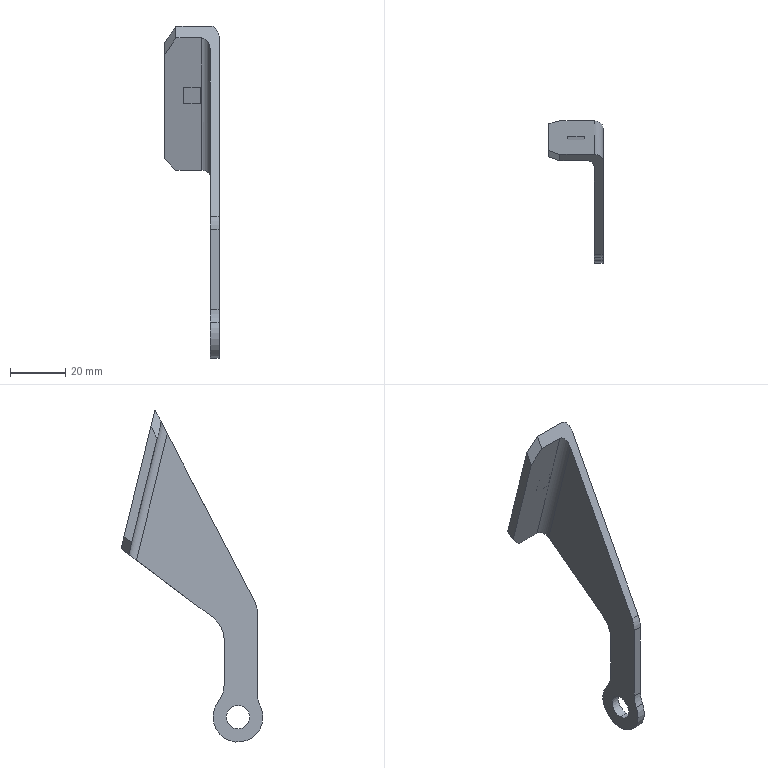Part | SolidWorks | features BaseBody 1 | 1 solid | 25 faces | box 19.6 x 51.2 x 119.9 mm | volume 9496 mm3 | plane 16 | cylinder 9 | commonest cylinder face diameters 20 x4 6.4 x2 8.479 x2 18 x1
STEP:
#1=CARTESIAN_POINT('',(1.6,0.,4.239));
#2=VERTEX_POINT('',#1);
#3=CARTESIAN_POINT('',(1.6,0.,-4.239));
#4=VERTEX_POINT('',#3);
#5=CARTESIAN_POINT('',(1.6,0.,0.));
#6=DIRECTION('',(1.,0.,0.));
#7=DIRECTION('',(0.,0.,1.));
#8=AXIS2_PLACEMENT_3D('',#5,#6,#7);
#9=CIRCLE('',#8,4.239);
#10=EDGE_CURVE('',#2,#4,#9,.T.);
#11=ORIENTED_EDGE('',*,*,#10,.T.);
#12=CARTESIAN_POINT('',(-1.6,0.,-4.239));
#13=VERTEX_POINT('',#12);
#14=CARTESIAN_POINT('',(1.6,0.,-4.239));
#15=DIRECTION('',(-1.,0.,0.));
#16=VECTOR('',#15,1000.);
#17=LINE('',#14,#16);
#18=EDGE_CURVE('',#4,#13,#17,.T.);
#19=ORIENTED_EDGE('',*,*,#18,.T.);
#20=CARTESIAN_POINT('',(-1.6,0.,4.239));
#21=VERTEX_POINT('',#20);
#22=CARTESIAN_POINT('',(-1.6,0.,0.));
#23=DIRECTION('',(-1.,0.,0.));
#24=DIRECTION('',(0.,0.,1.));
#25=AXIS2_PLACEMENT_3D('',#22,#23,#24);
#26=CIRCLE('',#25,4.239);
#27=EDGE_CURVE('',#13,#21,#26,.T.);
#28=ORIENTED_EDGE('',*,*,#27,.T.);
#29=CARTESIAN_POINT('',(1.6,0.,4.239));
#30=DIRECTION('',(-1.,0.,0.));
#31=VECTOR('',#30,1000.);
#32=LINE('',#29,#31);
#33=EDGE_CURVE('',#2,#21,#32,.T.);
#34=ORIENTED_EDGE('',*,*,#33,.F.);
#35=EDGE_LOOP('',(#11,#19,#28,#34));
#36=FACE_OUTER_BOUND('',#35,.T.);
#37=CARTESIAN_POINT('',(1.6,0.,0.));
#38=DIRECTION('',(-1.,0.,0.));
#39=DIRECTION('',(0.,0.,1.));
#40=AXIS2_PLACEMENT_3D('',#37,#38,#39);
#41=CYLINDRICAL_SURFACE('',#40,4.239);
#42=ADVANCED_FACE('',(#36),#41,.F.);
#43=ORIENTED_EDGE('',*,*,#18,.F.);
#44=CARTESIAN_POINT('',(1.6,0.,0.));
#45=DIRECTION('',(1.,0.,0.));
#46=DIRECTION('',(0.,0.,1.));
#47=AXIS2_PLACEMENT_3D('',#44,#45,#46);
#48=CIRCLE('',#47,4.239);
#49=EDGE_CURVE('',#4,#2,#48,.T.);
#50=ORIENTED_EDGE('',*,*,#49,.T.);
#51=ORIENTED_EDGE('',*,*,#33,.T.);
#52=CARTESIAN_POINT('',(-1.6,0.,0.));
#53=DIRECTION('',(-1.,0.,0.));
#54=DIRECTION('',(0.,0.,1.));
#55=AXIS2_PLACEMENT_3D('',#52,#53,#54);
#56=CIRCLE('',#55,4.239);
#57=EDGE_CURVE('',#21,#13,#56,.T.);
#58=ORIENTED_EDGE('',*,*,#57,.T.);
#59=EDGE_LOOP('',(#43,#50,#51,#58));
#60=FACE_OUTER_BOUND('',#59,.T.);
#61=CARTESIAN_POINT('',(1.6,0.,0.));
#62=DIRECTION('',(-1.,0.,0.));
#63=DIRECTION('',(0.,0.,1.));
#64=AXIS2_PLACEMENT_3D('',#61,#62,#63);
#65=CYLINDRICAL_SURFACE('',#64,4.239);
#66=ADVANCED_FACE('',(#60),#65,.F.);
#67=ORIENTED_EDGE('',*,*,#57,.F.);
#68=ORIENTED_EDGE('',*,*,#27,.F.);
#69=EDGE_LOOP('',(#67,#68));
#70=FACE_BOUND('',#69,.T.);
#71=CARTESIAN_POINT('',(-1.6,-7.,8.485));
#72=VERTEX_POINT('',#71);
#73=CARTESIAN_POINT('',(-1.6,-7.,37.451));
#74=VERTEX_POINT('',#73);
#75=CARTESIAN_POINT('',(-1.6,-7.,46.645));
#76=DIRECTION('',(0.,0.,1.));
#77=VECTOR('',#76,1000.);
#78=LINE('',#75,#77);
#79=EDGE_CURVE('',#72,#74,#78,.T.);
#80=ORIENTED_EDGE('',*,*,#79,.T.);
#81=CARTESIAN_POINT('',(-1.6,-5.868,42.072));
#82=VERTEX_POINT('',#81);
#83=CARTESIAN_POINT('',(-1.6,3.,37.451));
#84=DIRECTION('',(-1.,0.,0.));
#85=DIRECTION('',(0.,0.,1.));
#86=AXIS2_PLACEMENT_3D('',#83,#84,#85);
#87=CIRCLE('',#86,10.);
#88=EDGE_CURVE('',#74,#82,#87,.T.);
#89=ORIENTED_EDGE('',*,*,#88,.T.);
#90=CARTESIAN_POINT('',(-1.6,25.513,102.29));
#91=VERTEX_POINT('',#90);
#92=CARTESIAN_POINT('',(-1.6,-5.868,42.072));
#93=DIRECTION('',(0.,0.4621,0.8868));
#94=VECTOR('',#93,1000.);
#95=LINE('',#92,#94);
#96=EDGE_CURVE('',#82,#91,#95,.T.);
#97=ORIENTED_EDGE('',*,*,#96,.T.);
#98=CARTESIAN_POINT('',(-1.6,36.634,56.711));
#99=VERTEX_POINT('',#98);
#100=CARTESIAN_POINT('',(-1.6,25.513,102.29));
#101=DIRECTION('',(0.,0.237,-0.9715));
#102=VECTOR('',#101,1000.);
#103=LINE('',#100,#102);
#104=EDGE_CURVE('',#91,#99,#103,.T.);
#105=ORIENTED_EDGE('',*,*,#104,.T.);
#106=CARTESIAN_POINT('',(-1.6,8.986,35.9));
#107=VERTEX_POINT('',#106);
#108=CARTESIAN_POINT('',(-1.6,36.634,56.711));
#109=DIRECTION('',(0.,-0.799,-0.6014));
#110=VECTOR('',#109,1000.);
#111=LINE('',#108,#110);
#112=EDGE_CURVE('',#99,#107,#111,.T.);
#113=ORIENTED_EDGE('',*,*,#112,.T.);
#114=CARTESIAN_POINT('',(-1.6,5.,27.911));
#115=VERTEX_POINT('',#114);
#116=CARTESIAN_POINT('',(-1.6,15.,27.911));
#117=DIRECTION('',(1.,0.,0.));
#118=DIRECTION('',(0.,0.,1.));
#119=AXIS2_PLACEMENT_3D('',#116,#117,#118);
#120=CIRCLE('',#119,10.);
#121=EDGE_CURVE('',#107,#115,#120,.T.);
#122=ORIENTED_EDGE('',*,*,#121,.T.);
#123=CARTESIAN_POINT('',(-1.6,5.,11.662));
#124=VERTEX_POINT('',#123);
#125=CARTESIAN_POINT('',(-1.6,5.,46.645));
#126=DIRECTION('',(0.,0.,-1.));
#127=VECTOR('',#126,1000.);
#128=LINE('',#125,#127);
#129=EDGE_CURVE('',#115,#124,#128,.T.);
#130=ORIENTED_EDGE('',*,*,#129,.T.);
#131=CARTESIAN_POINT('',(-1.6,7.105,5.524));
#132=VERTEX_POINT('',#131);
#133=CARTESIAN_POINT('',(-1.6,15.,11.662));
#134=DIRECTION('',(1.,0.,0.));
#135=DIRECTION('',(0.,0.,1.));
#136=AXIS2_PLACEMENT_3D('',#133,#134,#135);
#137=CIRCLE('',#136,10.);
#138=EDGE_CURVE('',#124,#132,#137,.T.);
#139=ORIENTED_EDGE('',*,*,#138,.T.);
#140=CARTESIAN_POINT('',(-1.6,-8.053,4.019));
#141=VERTEX_POINT('',#140);
#142=CARTESIAN_POINT('',(-1.6,0.,0.));
#143=DIRECTION('',(-1.,0.,0.));
#144=DIRECTION('',(0.,0.,1.));
#145=AXIS2_PLACEMENT_3D('',#142,#143,#144);
#146=CIRCLE('',#145,9.);
#147=EDGE_CURVE('',#132,#141,#146,.T.);
#148=ORIENTED_EDGE('',*,*,#147,.T.);
#149=CARTESIAN_POINT('',(-1.6,-17.,8.485));
#150=DIRECTION('',(1.,0.,0.));
#151=DIRECTION('',(0.,0.,1.));
#152=AXIS2_PLACEMENT_3D('',#149,#150,#151);
#153=CIRCLE('',#152,10.);
#154=EDGE_CURVE('',#141,#72,#153,.T.);
#155=ORIENTED_EDGE('',*,*,#154,.T.);
#156=EDGE_LOOP('',(#80,#89,#97,#105,#113,#122,#130,#139,#148,#155));
#157=FACE_OUTER_BOUND('',#156,.T.);
#158=CARTESIAN_POINT('',(-1.6,-9.274,-9.668));
#159=DIRECTION('',(-1.,0.,0.));
#160=DIRECTION('',(0.,0.,1.));
#161=AXIS2_PLACEMENT_3D('',#158,#159,#160);
#162=PLANE('',#161);
#163=ADVANCED_FACE('',(#70,#157),#162,.T.);
#164=ORIENTED_EDGE('',*,*,#10,.F.);
#165=ORIENTED_EDGE('',*,*,#49,.F.);
#166=EDGE_LOOP('',(#164,#165));
#167=FACE_BOUND('',#166,.T.);
#168=CARTESIAN_POINT('',(1.6,27.757,106.595));
#169=VERTEX_POINT('',#168);
#170=CARTESIAN_POINT('',(1.6,39.417,58.805));
#171=VERTEX_POINT('',#170);
#172=CARTESIAN_POINT('',(1.6,39.492,58.497));
#173=DIRECTION('',(0.,0.237,-0.9715));
#174=VECTOR('',#173,1000.);
#175=LINE('',#172,#174);
#176=EDGE_CURVE('',#169,#171,#175,.T.);
#177=ORIENTED_EDGE('',*,*,#176,.F.);
#178=CARTESIAN_POINT('',(1.6,-5.868,42.072));
#179=VERTEX_POINT('',#178);
#180=CARTESIAN_POINT('',(1.6,-5.868,42.072));
#181=DIRECTION('',(0.,0.4621,0.8868));
#182=VECTOR('',#181,1000.);
#183=LINE('',#180,#182);
#184=EDGE_CURVE('',#179,#169,#183,.T.);
#185=ORIENTED_EDGE('',*,*,#184,.F.);
#186=CARTESIAN_POINT('',(1.6,-7.,37.451));
#187=VERTEX_POINT('',#186);
#188=CARTESIAN_POINT('',(1.6,3.,37.451));
#189=DIRECTION('',(-1.,0.,0.));
#190=DIRECTION('',(0.,0.,1.));
#191=AXIS2_PLACEMENT_3D('',#188,#189,#190);
#192=CIRCLE('',#191,10.);
#193=EDGE_CURVE('',#187,#179,#192,.T.);
#194=ORIENTED_EDGE('',*,*,#193,.F.);
#195=CARTESIAN_POINT('',(1.6,-7.,8.485));
#196=VERTEX_POINT('',#195);
#197=CARTESIAN_POINT('',(1.6,-7.,48.797));
#198=DIRECTION('',(0.,0.,1.));
#199=VECTOR('',#198,1000.);
#200=LINE('',#197,#199);
#201=EDGE_CURVE('',#196,#187,#200,.T.);
#202=ORIENTED_EDGE('',*,*,#201,.F.);
#203=CARTESIAN_POINT('',(1.6,-8.053,4.019));
#204=VERTEX_POINT('',#203);
#205=CARTESIAN_POINT('',(1.6,-17.,8.485));
#206=DIRECTION('',(1.,0.,0.));
#207=DIRECTION('',(0.,0.,1.));
#208=AXIS2_PLACEMENT_3D('',#205,#206,#207);
#209=CIRCLE('',#208,10.);
#210=EDGE_CURVE('',#204,#196,#209,.T.);
#211=ORIENTED_EDGE('',*,*,#210,.F.);
#212=CARTESIAN_POINT('',(1.6,7.105,5.524));
#213=VERTEX_POINT('',#212);
#214=CARTESIAN_POINT('',(1.6,0.,0.));
#215=DIRECTION('',(-1.,0.,0.));
#216=DIRECTION('',(0.,0.,1.));
#217=AXIS2_PLACEMENT_3D('',#214,#215,#216);
#218=CIRCLE('',#217,9.);
#219=EDGE_CURVE('',#213,#204,#218,.T.);
#220=ORIENTED_EDGE('',*,*,#219,.F.);
#221=CARTESIAN_POINT('',(1.6,5.,11.662));
#222=VERTEX_POINT('',#221);
#223=CARTESIAN_POINT('',(1.6,15.,11.662));
#224=DIRECTION('',(1.,0.,0.));
#225=DIRECTION('',(0.,0.,1.));
#226=AXIS2_PLACEMENT_3D('',#223,#224,#225);
#227=CIRCLE('',#226,10.);
#228=EDGE_CURVE('',#222,#213,#227,.T.);
#229=ORIENTED_EDGE('',*,*,#228,.F.);
#230=CARTESIAN_POINT('',(1.6,5.,27.911));
#231=VERTEX_POINT('',#230);
#232=CARTESIAN_POINT('',(1.6,5.,48.797));
#233=DIRECTION('',(0.,0.,-1.));
#234=VECTOR('',#233,1000.);
#235=LINE('',#232,#234);
#236=EDGE_CURVE('',#231,#222,#235,.T.);
#237=ORIENTED_EDGE('',*,*,#236,.F.);
#238=CARTESIAN_POINT('',(1.6,8.986,35.9));
#239=VERTEX_POINT('',#238);
#240=CARTESIAN_POINT('',(1.6,15.,27.911));
#241=DIRECTION('',(1.,0.,0.));
#242=DIRECTION('',(0.,0.,1.));
#243=AXIS2_PLACEMENT_3D('',#240,#241,#242);
#244=CIRCLE('',#243,10.);
#245=EDGE_CURVE('',#239,#231,#244,.T.);
#246=ORIENTED_EDGE('',*,*,#245,.F.);
#247=CARTESIAN_POINT('',(1.6,42.2,60.9));
#248=DIRECTION('',(0.,-0.799,-0.6014));
#249=VECTOR('',#248,1000.);
#250=LINE('',#247,#249);
#251=EDGE_CURVE('',#171,#239,#250,.T.);
#252=ORIENTED_EDGE('',*,*,#251,.F.);
#253=EDGE_LOOP('',(#177,#185,#194,#202,#211,#220,#229,#237,#246,#252));
#254=FACE_OUTER_BOUND('',#253,.T.);
#255=CARTESIAN_POINT('',(1.6,-9.291,-9.694));
#256=DIRECTION('',(-1.,0.,0.));
#257=DIRECTION('',(0.,0.,1.));
#258=AXIS2_PLACEMENT_3D('',#255,#256,#257);
#259=PLANE('',#258);
#260=ADVANCED_FACE('',(#167,#254),#259,.F.);
#261=CARTESIAN_POINT('',(0.,-7.,37.451));
#262=DIRECTION('',(-1.,0.,0.));
#263=VECTOR('',#262,1000.);
#264=LINE('',#261,#263);
#265=EDGE_CURVE('',#187,#74,#264,.T.);
#266=ORIENTED_EDGE('',*,*,#265,.F.);
#267=ORIENTED_EDGE('',*,*,#193,.T.);
#268=CARTESIAN_POINT('',(0.,-5.868,42.072));
#269=DIRECTION('',(1.,0.,0.));
#270=VECTOR('',#269,1000.);
#271=LINE('',#268,#270);
#272=EDGE_CURVE('',#82,#179,#271,.T.);
#273=ORIENTED_EDGE('',*,*,#272,.F.);
#274=ORIENTED_EDGE('',*,*,#88,.F.);
#275=EDGE_LOOP('',(#266,#267,#273,#274));
#276=FACE_OUTER_BOUND('',#275,.T.);
#277=CARTESIAN_POINT('',(1.6,3.,37.451));
#278=DIRECTION('',(-1.,0.,0.));
#279=DIRECTION('',(0.,0.,1.));
#280=AXIS2_PLACEMENT_3D('',#277,#278,#279);
#281=CYLINDRICAL_SURFACE('',#280,10.);
#282=ADVANCED_FACE('',(#276),#281,.T.);
#283=CARTESIAN_POINT('',(0.,-7.,8.485));
#284=DIRECTION('',(-1.,0.,0.));
#285=VECTOR('',#284,1000.);
#286=LINE('',#283,#285);
#287=EDGE_CURVE('',#196,#72,#286,.T.);
#288=ORIENTED_EDGE('',*,*,#287,.F.);
#289=ORIENTED_EDGE('',*,*,#201,.T.);
#290=ORIENTED_EDGE('',*,*,#265,.T.);
#291=ORIENTED_EDGE('',*,*,#79,.F.);
#292=EDGE_LOOP('',(#288,#289,#290,#291));
#293=FACE_OUTER_BOUND('',#292,.T.);
#294=CARTESIAN_POINT('',(-1.6,-7.,8.485));
#295=DIRECTION('',(0.,1.,0.));
#296=DIRECTION('',(0.,0.,1.));
#297=AXIS2_PLACEMENT_3D('',#294,#295,#296);
#298=PLANE('',#297);
#299=ADVANCED_FACE('',(#293),#298,.F.);
#300=ORIENTED_EDGE('',*,*,#210,.T.);
#301=ORIENTED_EDGE('',*,*,#287,.T.);
#302=ORIENTED_EDGE('',*,*,#154,.F.);
#303=CARTESIAN_POINT('',(0.,-8.053,4.019));
#304=DIRECTION('',(1.,0.,0.));
#305=VECTOR('',#304,1000.);
#306=LINE('',#303,#305);
#307=EDGE_CURVE('',#141,#204,#306,.T.);
#308=ORIENTED_EDGE('',*,*,#307,.T.);
#309=EDGE_LOOP('',(#300,#301,#302,#308));
#310=FACE_OUTER_BOUND('',#309,.T.);
#311=CARTESIAN_POINT('',(1.6,-17.,8.485));
#312=DIRECTION('',(-1.,0.,0.));
#313=DIRECTION('',(0.,0.,1.));
#314=AXIS2_PLACEMENT_3D('',#311,#312,#313);
#315=CYLINDRICAL_SURFACE('',#314,10.);
#316=ADVANCED_FACE('',(#310),#315,.F.);
#317=CARTESIAN_POINT('',(0.,7.105,5.524));
#318=DIRECTION('',(-1.,0.,0.));
#319=VECTOR('',#318,1000.);
#320=LINE('',#317,#319);
#321=EDGE_CURVE('',#213,#132,#320,.T.);
#322=ORIENTED_EDGE('',*,*,#321,.F.);
#323=ORIENTED_EDGE('',*,*,#219,.T.);
#324=ORIENTED_EDGE('',*,*,#307,.F.);
#325=ORIENTED_EDGE('',*,*,#147,.F.);
#326=EDGE_LOOP('',(#322,#323,#324,#325));
#327=FACE_OUTER_BOUND('',#326,.T.);
#328=CARTESIAN_POINT('',(1.6,0.,0.));
#329=DIRECTION('',(-1.,0.,0.));
#330=DIRECTION('',(0.,0.,1.));
#331=AXIS2_PLACEMENT_3D('',#328,#329,#330);
#332=CYLINDRICAL_SURFACE('',#331,9.);
#333=ADVANCED_FACE('',(#327),#332,.T.);
#334=ORIENTED_EDGE('',*,*,#228,.T.);
#335=ORIENTED_EDGE('',*,*,#321,.T.);
#336=ORIENTED_EDGE('',*,*,#138,.F.);
#337=CARTESIAN_POINT('',(0.,5.,11.662));
#338=DIRECTION('',(1.,0.,0.));
#339=VECTOR('',#338,1000.);
#340=LINE('',#337,#339);
#341=EDGE_CURVE('',#124,#222,#340,.T.);
#342=ORIENTED_EDGE('',*,*,#341,.T.);
#343=EDGE_LOOP('',(#334,#335,#336,#342));
#344=FACE_OUTER_BOUND('',#343,.T.);
#345=CARTESIAN_POINT('',(1.6,15.,11.662));
#346=DIRECTION('',(-1.,0.,0.));
#347=DIRECTION('',(0.,0.,1.));
#348=AXIS2_PLACEMENT_3D('',#345,#346,#347);
#349=CYLINDRICAL_SURFACE('',#348,10.);
#350=ADVANCED_FACE('',(#344),#349,.F.);
#351=CARTESIAN_POINT('',(0.,5.,27.911));
#352=DIRECTION('',(-1.,0.,0.));
#353=VECTOR('',#352,1000.);
#354=LINE('',#351,#353);
#355=EDGE_CURVE('',#231,#115,#354,.T.);
#356=ORIENTED_EDGE('',*,*,#355,.F.);
#357=ORIENTED_EDGE('',*,*,#236,.T.);
#358=ORIENTED_EDGE('',*,*,#341,.F.);
#359=ORIENTED_EDGE('',*,*,#129,.F.);
#360=EDGE_LOOP('',(#356,#357,#358,#359));
#361=FACE_OUTER_BOUND('',#360,.T.);
#362=CARTESIAN_POINT('',(-1.6,5.,27.911));
#363=DIRECTION('',(0.,-1.,0.));
#364=DIRECTION('',(0.,0.,-1.));
#365=AXIS2_PLACEMENT_3D('',#362,#363,#364);
#366=PLANE('',#365);
#367=ADVANCED_FACE('',(#361),#366,.F.);
#368=ORIENTED_EDGE('',*,*,#245,.T.);
#369=ORIENTED_EDGE('',*,*,#355,.T.);
#370=ORIENTED_EDGE('',*,*,#121,.F.);
#371=CARTESIAN_POINT('',(0.,8.986,35.9));
#372=DIRECTION('',(1.,0.,0.));
#373=VECTOR('',#372,1000.);
#374=LINE('',#371,#373);
#375=EDGE_CURVE('',#107,#239,#374,.T.);
#376=ORIENTED_EDGE('',*,*,#375,.T.);
#377=EDGE_LOOP('',(#368,#369,#370,#376));
#378=FACE_OUTER_BOUND('',#377,.T.);
#379=CARTESIAN_POINT('',(1.6,15.,27.911));
#380=DIRECTION('',(-1.,0.,0.));
#381=DIRECTION('',(0.,0.,1.));
#382=AXIS2_PLACEMENT_3D('',#379,#380,#381);
#383=CYLINDRICAL_SURFACE('',#382,10.);
#384=ADVANCED_FACE('',(#378),#383,.F.);
#385=CARTESIAN_POINT('',(-1.6,42.2,60.9));
#386=VERTEX_POINT('',#385);
#387=CARTESIAN_POINT('',(1.6,39.417,58.805));
#388=CARTESIAN_POINT('',(1.6,41.047,60.032));
#389=CARTESIAN_POINT('',(0.2745,42.2,60.9));
#390=CARTESIAN_POINT('',(-1.6,42.2,60.9));
#391=(BOUNDED_CURVE()B_SPLINE_CURVE(3,(#387,#388,#389,#390),.UNSPECIFIED.,.F.,.F.)B_SPLINE_CURVE_WITH_KNOTS((4,4),(4.712,6.283),.UNSPECIFIED.)CURVE()GEOMETRIC_REPRESENTATION_ITEM()RATIONAL_B_SPLINE_CURVE((1.,0.8047,0.8047,1.))REPRESENTATION_ITEM(''));
#392=EDGE_CURVE('',#171,#386,#391,.T.);
#393=ORIENTED_EDGE('',*,*,#392,.F.);
#394=ORIENTED_EDGE('',*,*,#251,.T.);
#395=ORIENTED_EDGE('',*,*,#375,.F.);
#396=ORIENTED_EDGE('',*,*,#112,.F.);
#397=CARTESIAN_POINT('',(-4.8,39.417,58.805));
#398=VERTEX_POINT('',#397);
#399=CARTESIAN_POINT('',(-4.8,39.417,58.805));
#400=CARTESIAN_POINT('',(-2.925,39.417,58.805));
#401=CARTESIAN_POINT('',(-1.6,38.265,57.938));
#402=CARTESIAN_POINT('',(-1.6,36.634,56.711));
#403=(BOUNDED_CURVE()B_SPLINE_CURVE(3,(#399,#400,#401,#402),.UNSPECIFIED.,.F.,.F.)B_SPLINE_CURVE_WITH_KNOTS((4,4),(6.283,7.854),.UNSPECIFIED.)CURVE()GEOMETRIC_REPRESENTATION_ITEM()RATIONAL_B_SPLINE_CURVE((1.,0.8047,0.8047,1.))REPRESENTATION_ITEM(''));
#404=EDGE_CURVE('',#398,#99,#403,.T.);
#405=ORIENTED_EDGE('',*,*,#404,.F.);
#406=CARTESIAN_POINT('',(-14.,39.417,58.805));
#407=VERTEX_POINT('',#406);
#408=CARTESIAN_POINT('',(-6.2,39.417,58.805));
#409=DIRECTION('',(1.,0.,0.));
#410=VECTOR('',#409,1000.);
#411=LINE('',#408,#410);
#412=EDGE_CURVE('',#407,#398,#411,.T.);
#413=ORIENTED_EDGE('',*,*,#412,.F.);
#414=CARTESIAN_POINT('',(-14.,42.2,60.9));
#415=VERTEX_POINT('',#414);
#416=CARTESIAN_POINT('',(-14.,25.593,48.4));
#417=DIRECTION('',(0.,-0.799,-0.6014));
#418=VECTOR('',#417,1000.);
#419=LINE('',#416,#418);
#420=EDGE_CURVE('',#415,#407,#419,.T.);
#421=ORIENTED_EDGE('',*,*,#420,.F.);
#422=CARTESIAN_POINT('',(-6.2,42.2,60.9));
#423=DIRECTION('',(-1.,0.,0.));
#424=VECTOR('',#423,1000.);
#425=LINE('',#422,#424);
#426=EDGE_CURVE('',#386,#415,#425,.T.);
#427=ORIENTED_EDGE('',*,*,#426,.F.);
#428=EDGE_LOOP('',(#393,#394,#395,#396,#405,#413,#421,#427));
#429=FACE_OUTER_BOUND('',#428,.T.);
#430=CARTESIAN_POINT('',(-14.,42.2,60.9));
#431=DIRECTION('',(0.,-0.6014,0.799));
#432=DIRECTION('',(0.,-0.799,-0.6014));
#433=AXIS2_PLACEMENT_3D('',#430,#431,#432);
#434=PLANE('',#433);
#435=ADVANCED_FACE('',(#429),#434,.F.);
#436=CARTESIAN_POINT('',(-4.8,27.757,106.595));
#437=VERTEX_POINT('',#436);
#438=CARTESIAN_POINT('',(-1.6,25.513,102.29));
#439=CARTESIAN_POINT('',(-1.6,26.827,104.812));
#440=CARTESIAN_POINT('',(-2.925,27.757,106.595));
#441=CARTESIAN_POINT('',(-4.8,27.757,106.595));
#442=(BOUNDED_CURVE()B_SPLINE_CURVE(3,(#438,#439,#440,#441),.UNSPECIFIED.,.F.,.F.)B_SPLINE_CURVE_WITH_KNOTS((4,4),(4.712,6.283),.UNSPECIFIED.)CURVE()GEOMETRIC_REPRESENTATION_ITEM()RATIONAL_B_SPLINE_CURVE((1.,0.8047,0.8047,1.))REPRESENTATION_ITEM(''));
#443=EDGE_CURVE('',#91,#437,#442,.T.);
#444=ORIENTED_EDGE('',*,*,#443,.T.);
#445=CARTESIAN_POINT('',(-4.8,33.75,82.032));
#446=DIRECTION('',(0.,0.237,-0.9715));
#447=VECTOR('',#446,1000.);
#448=LINE('',#445,#447);
#449=EDGE_CURVE('',#437,#398,#448,.T.);
#450=ORIENTED_EDGE('',*,*,#449,.T.);
#451=ORIENTED_EDGE('',*,*,#404,.T.);
#452=ORIENTED_EDGE('',*,*,#104,.F.);
#453=EDGE_LOOP('',(#444,#450,#451,#452));
#454=FACE_OUTER_BOUND('',#453,.T.);
#455=CARTESIAN_POINT('',(-4.8,36.706,56.416));
#456=DIRECTION('',(0.,-0.237,0.9715));
#457=DIRECTION('',(0.,-0.9715,-0.237));
#458=AXIS2_PLACEMENT_3D('',#455,#456,#457);
#459=CYLINDRICAL_SURFACE('',#458,3.2);
#460=ADVANCED_FACE('',(#454),#459,.F.);
#461=CARTESIAN_POINT('',(-1.6,30.,110.9));
#462=VERTEX_POINT('',#461);
#463=CARTESIAN_POINT('',(-1.6,30.,110.9));
#464=CARTESIAN_POINT('',(0.2745,30.,110.9));
#465=CARTESIAN_POINT('',(1.6,29.071,109.117));
#466=CARTESIAN_POINT('',(1.6,27.757,106.595));
#467=(BOUNDED_CURVE()B_SPLINE_CURVE(3,(#463,#464,#465,#466),.UNSPECIFIED.,.F.,.F.)B_SPLINE_CURVE_WITH_KNOTS((4,4),(6.283,7.854),.UNSPECIFIED.)CURVE()GEOMETRIC_REPRESENTATION_ITEM()RATIONAL_B_SPLINE_CURVE((1.,0.8047,0.8047,1.))REPRESENTATION_ITEM(''));
#468=EDGE_CURVE('',#462,#169,#467,.T.);
#469=ORIENTED_EDGE('',*,*,#468,.F.);
#470=CARTESIAN_POINT('',(-14.,30.,110.9));
#471=VERTEX_POINT('',#470);
#472=CARTESIAN_POINT('',(-6.2,30.,110.9));
#473=DIRECTION('',(1.,0.,0.));
#474=VECTOR('',#473,1000.);
#475=LINE('',#472,#474);
#476=EDGE_CURVE('',#471,#462,#475,.T.);
#477=ORIENTED_EDGE('',*,*,#476,.F.);
#478=CARTESIAN_POINT('',(-14.,27.757,106.595));
#479=VERTEX_POINT('',#478);
#480=CARTESIAN_POINT('',(-14.,12.066,76.486));
#481=DIRECTION('',(0.,0.4621,0.8868));
#482=VECTOR('',#481,1000.);
#483=LINE('',#480,#482);
#484=EDGE_CURVE('',#479,#471,#483,.T.);
#485=ORIENTED_EDGE('',*,*,#484,.F.);
#486=CARTESIAN_POINT('',(-6.2,27.757,106.595));
#487=DIRECTION('',(-1.,0.,0.));
#488=VECTOR('',#487,1000.);
#489=LINE('',#486,#488);
#490=EDGE_CURVE('',#437,#479,#489,.T.);
#491=ORIENTED_EDGE('',*,*,#490,.F.);
#492=ORIENTED_EDGE('',*,*,#443,.F.);
#493=ORIENTED_EDGE('',*,*,#96,.F.);
#494=ORIENTED_EDGE('',*,*,#272,.T.);
#495=ORIENTED_EDGE('',*,*,#184,.T.);
#496=EDGE_LOOP('',(#469,#477,#485,#491,#492,#493,#494,#495));
#497=FACE_OUTER_BOUND('',#496,.T.);
#498=CARTESIAN_POINT('',(-14.,-5.868,42.072));
#499=DIRECTION('',(0.,0.8868,-0.4621));
#500=DIRECTION('',(0.,0.4621,0.8868));
#501=AXIS2_PLACEMENT_3D('',#498,#499,#500);
#502=PLANE('',#501);
#503=ADVANCED_FACE('',(#497),#502,.F.);
#504=CARTESIAN_POINT('',(-1.6,36.263,85.232));
#505=DIRECTION('',(0.,0.237,-0.9715));
#506=VECTOR('',#505,1000.);
#507=LINE('',#504,#506);
#508=EDGE_CURVE('',#462,#386,#507,.T.);
#509=ORIENTED_EDGE('',*,*,#508,.F.);
#510=ORIENTED_EDGE('',*,*,#468,.T.);
#511=ORIENTED_EDGE('',*,*,#176,.T.);
#512=ORIENTED_EDGE('',*,*,#392,.T.);
#513=EDGE_LOOP('',(#509,#510,#511,#512));
#514=FACE_OUTER_BOUND('',#513,.T.);
#515=CARTESIAN_POINT('',(-1.6,39.492,58.497));
#516=DIRECTION('',(0.,-0.237,0.9715));
#517=DIRECTION('',(0.,-0.9715,-0.237));
#518=AXIS2_PLACEMENT_3D('',#515,#516,#517);
#519=CYLINDRICAL_SURFACE('',#518,3.2);
#520=ADVANCED_FACE('',(#514),#519,.T.);
#521=CARTESIAN_POINT('',(-11.2,36.638,83.693));
#522=VERTEX_POINT('',#521);
#523=CARTESIAN_POINT('',(-11.2,35.216,89.522));
#524=VERTEX_POINT('',#523);
#525=CARTESIAN_POINT('',(-11.2,36.1,85.9));
#526=DIRECTION('',(0.,-0.237,0.9715));
#527=VECTOR('',#526,1000.);
#528=LINE('',#525,#527);
#529=EDGE_CURVE('',#522,#524,#528,.T.);
#530=ORIENTED_EDGE('',*,*,#529,.F.);
#531=CARTESIAN_POINT('',(-5.2,36.638,83.693));
#532=VERTEX_POINT('',#531);
#533=CARTESIAN_POINT('',(-9.8,36.638,83.693));
#534=DIRECTION('',(-1.,0.,0.));
#535=VECTOR('',#534,1000.);
#536=LINE('',#533,#535);
#537=EDGE_CURVE('',#532,#522,#536,.T.);
#538=ORIENTED_EDGE('',*,*,#537,.F.);
#539=CARTESIAN_POINT('',(-5.2,35.216,89.522));
#540=VERTEX_POINT('',#539);
#541=CARTESIAN_POINT('',(-5.2,36.1,85.9));
#542=DIRECTION('',(0.,0.237,-0.9715));
#543=VECTOR('',#542,1000.);
#544=LINE('',#541,#543);
#545=EDGE_CURVE('',#540,#532,#544,.T.);
#546=ORIENTED_EDGE('',*,*,#545,.F.);
#547=CARTESIAN_POINT('',(-9.8,35.216,89.522));
#548=DIRECTION('',(1.,0.,0.));
#549=VECTOR('',#548,1000.);
#550=LINE('',#547,#549);
#551=EDGE_CURVE('',#524,#540,#550,.T.);
#552=ORIENTED_EDGE('',*,*,#551,.F.);
#553=EDGE_LOOP('',(#530,#538,#546,#552));
#554=FACE_BOUND('',#553,.T.);
#555=ORIENTED_EDGE('',*,*,#508,.T.);
#556=ORIENTED_EDGE('',*,*,#426,.T.);
#557=CARTESIAN_POINT('',(-18.,41.168,65.13));
#558=VERTEX_POINT('',#557);
#559=CARTESIAN_POINT('',(-18.,41.168,65.13));
#560=DIRECTION('',(0.6766,0.1746,-0.7154));
#561=VECTOR('',#560,1000.);
#562=LINE('',#559,#561);
#563=EDGE_CURVE('',#558,#415,#562,.T.);
#564=ORIENTED_EDGE('',*,*,#563,.F.);
#565=CARTESIAN_POINT('',(-18.,31.438,105.005));
#566=VERTEX_POINT('',#565);
#567=CARTESIAN_POINT('',(-18.,36.1,85.9));
#568=DIRECTION('',(0.,0.237,-0.9715));
#569=VECTOR('',#568,1000.);
#570=LINE('',#567,#569);
#571=EDGE_CURVE('',#566,#558,#570,.T.);
#572=ORIENTED_EDGE('',*,*,#571,.F.);
#573=CARTESIAN_POINT('',(-14.,30.,110.9));
#574=DIRECTION('',(-0.5504,0.1979,-0.8111));
#575=VECTOR('',#574,1000.);
#576=LINE('',#573,#575);
#577=EDGE_CURVE('',#471,#566,#576,.T.);
#578=ORIENTED_EDGE('',*,*,#577,.F.);
#579=ORIENTED_EDGE('',*,*,#476,.T.);
#580=EDGE_LOOP('',(#555,#556,#564,#572,#578,#579));
#581=FACE_OUTER_BOUND('',#580,.T.);
#582=CARTESIAN_POINT('',(-18.,30.,110.9));
#583=DIRECTION('',(0.,-0.9715,-0.237));
#584=DIRECTION('',(0.,0.237,-0.9715));
#585=AXIS2_PLACEMENT_3D('',#582,#583,#584);
#586=PLANE('',#585);
#587=ADVANCED_FACE('',(#554,#581),#586,.F.);
#588=ORIENTED_EDGE('',*,*,#449,.F.);
#589=ORIENTED_EDGE('',*,*,#490,.T.);
#590=CARTESIAN_POINT('',(-18.,29.195,100.7));
#591=VERTEX_POINT('',#590);
#592=CARTESIAN_POINT('',(-18.,29.195,100.7));
#593=DIRECTION('',(0.5504,-0.1979,0.8111));
#594=VECTOR('',#593,1000.);
#595=LINE('',#592,#594);
#596=EDGE_CURVE('',#591,#479,#595,.T.);
#597=ORIENTED_EDGE('',*,*,#596,.F.);
#598=CARTESIAN_POINT('',(-18.,38.385,63.035));
#599=VERTEX_POINT('',#598);
#600=CARTESIAN_POINT('',(-18.,33.587,82.7));
#601=DIRECTION('',(0.,-0.237,0.9715));
#602=VECTOR('',#601,1000.);
#603=LINE('',#600,#602);
#604=EDGE_CURVE('',#599,#591,#603,.T.);
#605=ORIENTED_EDGE('',*,*,#604,.F.);
#606=CARTESIAN_POINT('',(-14.,39.417,58.805));
#607=DIRECTION('',(-0.6766,-0.1746,0.7154));
#608=VECTOR('',#607,1000.);
#609=LINE('',#606,#608);
#610=EDGE_CURVE('',#407,#599,#609,.T.);
#611=ORIENTED_EDGE('',*,*,#610,.F.);
#612=ORIENTED_EDGE('',*,*,#412,.T.);
#613=EDGE_LOOP('',(#588,#589,#597,#605,#611,#612));
#614=FACE_OUTER_BOUND('',#613,.T.);
#615=CARTESIAN_POINT('',(-18.,39.417,58.805));
#616=DIRECTION('',(0.,0.9715,0.237));
#617=DIRECTION('',(0.,-0.237,0.9715));
#618=AXIS2_PLACEMENT_3D('',#615,#616,#617);
#619=PLANE('',#618);
#620=ADVANCED_FACE('',(#614),#619,.F.);
#621=ORIENTED_EDGE('',*,*,#420,.T.);
#622=ORIENTED_EDGE('',*,*,#610,.T.);
#623=CARTESIAN_POINT('',(-18.,41.168,65.13));
#624=DIRECTION('',(0.,-0.799,-0.6014));
#625=VECTOR('',#624,1000.);
#626=LINE('',#623,#625);
#627=EDGE_CURVE('',#558,#599,#626,.T.);
#628=ORIENTED_EDGE('',*,*,#627,.F.);
#629=ORIENTED_EDGE('',*,*,#563,.T.);
#630=EDGE_LOOP('',(#621,#622,#628,#629));
#631=FACE_OUTER_BOUND('',#630,.T.);
#632=CARTESIAN_POINT('',(-19.058,38.362,64.342));
#633=DIRECTION('',(0.7071,-0.4252,0.565));
#634=DIRECTION('',(0.6242,0.,-0.7813));
#635=AXIS2_PLACEMENT_3D('',#632,#633,#634);
#636=PLANE('',#635);
#637=ADVANCED_FACE('',(#631),#636,.F.);
#638=ORIENTED_EDGE('',*,*,#484,.T.);
#639=ORIENTED_EDGE('',*,*,#577,.T.);
#640=CARTESIAN_POINT('',(-18.,29.195,100.7));
#641=DIRECTION('',(0.,0.4621,0.8868));
#642=VECTOR('',#641,1000.);
#643=LINE('',#640,#642);
#644=EDGE_CURVE('',#591,#566,#643,.T.);
#645=ORIENTED_EDGE('',*,*,#644,.F.);
#646=ORIENTED_EDGE('',*,*,#596,.T.);
#647=EDGE_LOOP('',(#638,#639,#645,#646));
#648=FACE_OUTER_BOUND('',#647,.T.);
#649=CARTESIAN_POINT('',(-15.519,26.366,100.639));
#650=DIRECTION('',(0.7071,0.6271,-0.3268));
#651=DIRECTION('',(-0.6635,0.7482,0.));
#652=AXIS2_PLACEMENT_3D('',#649,#650,#651);
#653=PLANE('',#652);
#654=ADVANCED_FACE('',(#648),#653,.F.);
#655=CARTESIAN_POINT('',(-5.2,32.302,88.811));
#656=VERTEX_POINT('',#655);
#657=CARTESIAN_POINT('',(-5.2,33.759,89.167));
#658=DIRECTION('',(0.,0.9715,0.237));
#659=VECTOR('',#658,1000.);
#660=LINE('',#657,#659);
#661=EDGE_CURVE('',#656,#540,#660,.T.);
#662=ORIENTED_EDGE('',*,*,#661,.F.);
#663=CARTESIAN_POINT('',(-11.2,32.302,88.811));
#664=VERTEX_POINT('',#663);
#665=CARTESIAN_POINT('',(-8.2,32.302,88.811));
#666=DIRECTION('',(1.,0.,0.));
#667=VECTOR('',#666,1000.);
#668=LINE('',#665,#667);
#669=EDGE_CURVE('',#664,#656,#668,.T.);
#670=ORIENTED_EDGE('',*,*,#669,.F.);
#671=CARTESIAN_POINT('',(-11.2,33.759,89.167));
#672=DIRECTION('',(0.,-0.9715,-0.237));
#673=VECTOR('',#672,1000.);
#674=LINE('',#671,#673);
#675=EDGE_CURVE('',#524,#664,#674,.T.);
#676=ORIENTED_EDGE('',*,*,#675,.F.);
#677=ORIENTED_EDGE('',*,*,#551,.T.);
#678=EDGE_LOOP('',(#662,#670,#676,#677));
#679=FACE_OUTER_BOUND('',#678,.T.);
#680=CARTESIAN_POINT('',(-11.2,35.216,89.522));
#681=DIRECTION('',(0.,-0.237,0.9715));
#682=DIRECTION('',(0.,-0.9715,-0.237));
#683=AXIS2_PLACEMENT_3D('',#680,#681,#682);
#684=PLANE('',#683);
#685=ADVANCED_FACE('',(#679),#684,.F.);
#686=ORIENTED_EDGE('',*,*,#675,.T.);
#687=CARTESIAN_POINT('',(-11.2,33.724,82.982));
#688=VERTEX_POINT('',#687);
#689=CARTESIAN_POINT('',(-11.2,32.302,88.811));
#690=DIRECTION('',(0.,-0.237,0.9715));
#691=VECTOR('',#690,1000.);
#692=LINE('',#689,#691);
#693=EDGE_CURVE('',#688,#664,#692,.T.);
#694=ORIENTED_EDGE('',*,*,#693,.F.);
#695=CARTESIAN_POINT('',(-11.2,33.724,82.982));
#696=DIRECTION('',(0.,-0.9715,-0.237));
#697=VECTOR('',#696,1000.);
#698=LINE('',#695,#697);
#699=EDGE_CURVE('',#522,#688,#698,.T.);
#700=ORIENTED_EDGE('',*,*,#699,.F.);
#701=ORIENTED_EDGE('',*,*,#529,.T.);
#702=EDGE_LOOP('',(#686,#694,#700,#701));
#703=FACE_OUTER_BOUND('',#702,.T.);
#704=CARTESIAN_POINT('',(-11.2,32.276,82.943));
#705=DIRECTION('',(-1.,0.,0.));
#706=DIRECTION('',(0.,0.,1.));
#707=AXIS2_PLACEMENT_3D('',#704,#705,#706);
#708=PLANE('',#707);
#709=ADVANCED_FACE('',(#703),#708,.F.);
#710=ORIENTED_EDGE('',*,*,#699,.T.);
#711=CARTESIAN_POINT('',(-5.2,33.724,82.982));
#712=VERTEX_POINT('',#711);
#713=CARTESIAN_POINT('',(-8.2,33.724,82.982));
#714=DIRECTION('',(-1.,0.,0.));
#715=VECTOR('',#714,1000.);
#716=LINE('',#713,#715);
#717=EDGE_CURVE('',#712,#688,#716,.T.);
#718=ORIENTED_EDGE('',*,*,#717,.F.);
#719=CARTESIAN_POINT('',(-5.2,35.181,83.338));
#720=DIRECTION('',(0.,-0.9715,-0.237));
#721=VECTOR('',#720,1000.);
#722=LINE('',#719,#721);
#723=EDGE_CURVE('',#532,#712,#722,.T.);
#724=ORIENTED_EDGE('',*,*,#723,.F.);
#725=ORIENTED_EDGE('',*,*,#537,.T.);
#726=EDGE_LOOP('',(#710,#718,#724,#725));
#727=FACE_OUTER_BOUND('',#726,.T.);
#728=CARTESIAN_POINT('',(-11.2,33.724,82.982));
#729=DIRECTION('',(0.,0.237,-0.9715));
#730=DIRECTION('',(0.,0.9715,0.237));
#731=AXIS2_PLACEMENT_3D('',#728,#729,#730);
#732=PLANE('',#731);
#733=ADVANCED_FACE('',(#727),#732,.F.);
#734=ORIENTED_EDGE('',*,*,#723,.T.);
#735=CARTESIAN_POINT('',(-5.2,32.302,88.811));
#736=DIRECTION('',(0.,0.237,-0.9715));
#737=VECTOR('',#736,1000.);
#738=LINE('',#735,#737);
#739=EDGE_CURVE('',#656,#712,#738,.T.);
#740=ORIENTED_EDGE('',*,*,#739,.F.);
#741=ORIENTED_EDGE('',*,*,#661,.T.);
#742=ORIENTED_EDGE('',*,*,#545,.T.);
#743=EDGE_LOOP('',(#734,#740,#741,#742));
#744=FACE_OUTER_BOUND('',#743,.T.);
#745=CARTESIAN_POINT('',(-5.2,32.276,89.561));
#746=DIRECTION('',(1.,0.,0.));
#747=DIRECTION('',(0.,0.,-1.));
#748=AXIS2_PLACEMENT_3D('',#745,#746,#747);
#749=PLANE('',#748);
#750=ADVANCED_FACE('',(#744),#749,.F.);
#751=ORIENTED_EDGE('',*,*,#627,.T.);
#752=ORIENTED_EDGE('',*,*,#604,.T.);
#753=ORIENTED_EDGE('',*,*,#644,.T.);
#754=ORIENTED_EDGE('',*,*,#571,.T.);
#755=EDGE_LOOP('',(#751,#752,#753,#754));
#756=FACE_OUTER_BOUND('',#755,.T.);
#757=CARTESIAN_POINT('',(-18.,29.123,105.257));
#758=DIRECTION('',(1.,0.,0.));
#759=DIRECTION('',(0.,0.,-1.));
#760=AXIS2_PLACEMENT_3D('',#757,#758,#759);
#761=PLANE('',#760);
#762=ADVANCED_FACE('',(#756),#761,.F.);
#763=ORIENTED_EDGE('',*,*,#669,.T.);
#764=ORIENTED_EDGE('',*,*,#739,.T.);
#765=ORIENTED_EDGE('',*,*,#717,.T.);
#766=ORIENTED_EDGE('',*,*,#693,.T.);
#767=EDGE_LOOP('',(#763,#764,#765,#766));
#768=FACE_OUTER_BOUND('',#767,.T.);
#769=CARTESIAN_POINT('',(-11.2,32.302,88.811));
#770=DIRECTION('',(0.,-0.9715,-0.237));
#771=DIRECTION('',(0.,0.237,-0.9715));
#772=AXIS2_PLACEMENT_3D('',#769,#770,#771);
#773=PLANE('',#772);
#774=ADVANCED_FACE('',(#768),#773,.F.);
#775=CLOSED_SHELL('',(#42,#66,#163,#260,#282,#299,#316,#333,#350,#367,#384,#435,#460,#503,#520,#587,#620,#637,#654,#685,#709,#733,#750,#762,#774));
#776=MANIFOLD_SOLID_BREP('',#775);
#777=CARTESIAN_POINT('',(0.,0.,0.));
#778=DIRECTION('',(0.,0.,1.));
#779=DIRECTION('',(1.,0.,0.));
#780=AXIS2_PLACEMENT_3D('',#777,#778,#779);
#781=(LENGTH_UNIT()NAMED_UNIT(*)SI_UNIT(.MILLI.,.METRE.));
#782=UNCERTAINTY_MEASURE_WITH_UNIT(LENGTH_MEASURE(0.00001),#781,'','');
#783=(NAMED_UNIT(*)PLANE_ANGLE_UNIT()SI_UNIT($,.RADIAN.));
#784=(NAMED_UNIT(*)SI_UNIT($,.STERADIAN.)SOLID_ANGLE_UNIT());
#785=(GEOMETRIC_REPRESENTATION_CONTEXT(3)GLOBAL_UNCERTAINTY_ASSIGNED_CONTEXT((#782))GLOBAL_UNIT_ASSIGNED_CONTEXT((#781,#783,#784))REPRESENTATION_CONTEXT('',''));
#786=ADVANCED_BREP_SHAPE_REPRESENTATION('',(#776,#780),#785);